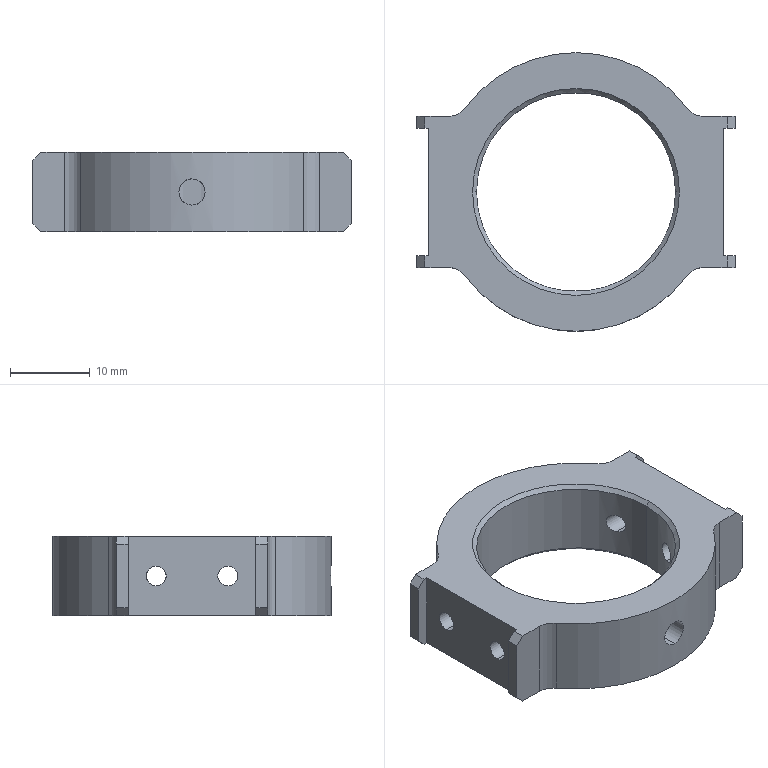Part | SolidWorks | features ICE 3, Chamfer 2, HoleWzd 2, Extrusion 1, Fillet 1, MirrorPattern 1 | 1 solid | 46 faces | box 40 x 35 x 10 mm | volume 5332 mm3 | plane 24 | cylinder 18 | cone 4 | commonest cylinder face diameters 2.5 x8 5 x4 3.3 x2 25 x2 35 x2